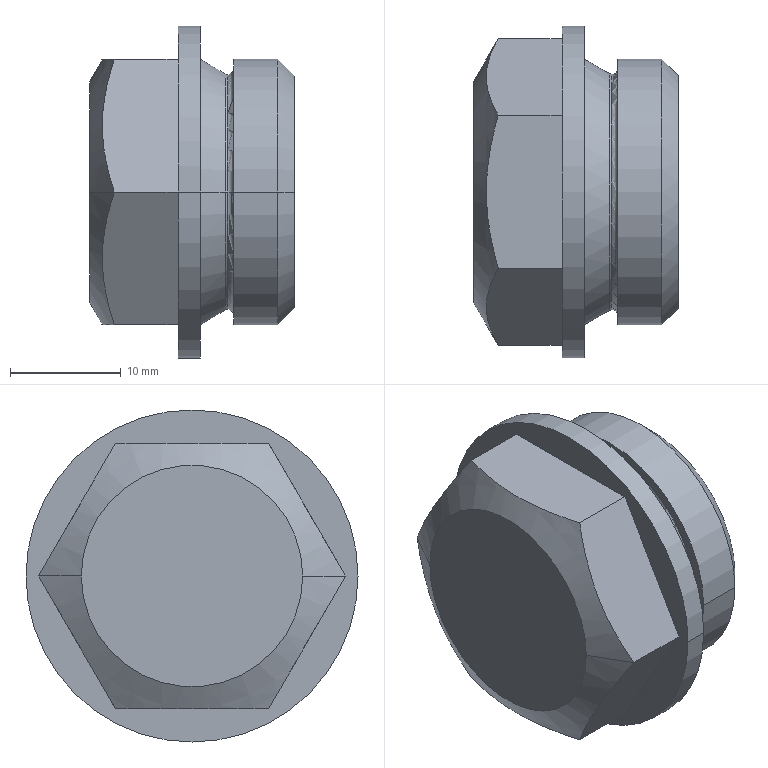Part | SolidWorks | features BaseBody 1 | 1 solid | 28 faces | box 18.5 x 30 x 30 mm | volume 4753 mm3 | plane 12 | cylinder 6 | cone 6 | torus 4 | commonest cylinder face diameters 17.5 x2 24 x2 30 x2
STEP:
#1=CARTESIAN_POINT('',(0.75,87.299,-16.));
#2=VERTEX_POINT('',#1);
#3=CARTESIAN_POINT('',(1.,87.366,-16.));
#4=VERTEX_POINT('',#3);
#5=CARTESIAN_POINT('',(1.,86.866,-16.));
#6=DIRECTION('',(0.,0.,-1.));
#7=DIRECTION('',(0.,1.,0.));
#8=AXIS2_PLACEMENT_3D('',#5,#6,#7);
#9=CIRCLE('',#8,0.5);
#10=EDGE_CURVE('',#2,#4,#9,.T.);
#11=ORIENTED_EDGE('',*,*,#10,.T.);
#12=CARTESIAN_POINT('',(1.,108.634,-16.));
#13=VERTEX_POINT('',#12);
#14=CARTESIAN_POINT('',(1.,98.,-16.));
#15=DIRECTION('',(-1.,0.,0.));
#16=DIRECTION('',(0.,-1.,0.));
#17=AXIS2_PLACEMENT_3D('',#14,#15,#16);
#18=CIRCLE('',#17,10.634);
#19=EDGE_CURVE('',#4,#13,#18,.T.);
#20=ORIENTED_EDGE('',*,*,#19,.T.);
#21=CARTESIAN_POINT('',(0.75,108.701,-16.));
#22=VERTEX_POINT('',#21);
#23=CARTESIAN_POINT('',(1.,109.134,-16.));
#24=DIRECTION('',(0.,0.,1.));
#25=DIRECTION('',(0.,-1.,0.));
#26=AXIS2_PLACEMENT_3D('',#23,#24,#25);
#27=CIRCLE('',#26,0.5);
#28=EDGE_CURVE('',#22,#13,#27,.T.);
#29=ORIENTED_EDGE('',*,*,#28,.F.);
#30=CARTESIAN_POINT('',(0.75,98.,-16.));
#31=DIRECTION('',(-1.,0.,0.));
#32=DIRECTION('',(0.,-1.,0.));
#33=AXIS2_PLACEMENT_3D('',#30,#31,#32);
#34=CIRCLE('',#33,10.701);
#35=EDGE_CURVE('',#2,#22,#34,.T.);
#36=ORIENTED_EDGE('',*,*,#35,.F.);
#37=EDGE_LOOP('',(#11,#20,#29,#36));
#38=FACE_OUTER_BOUND('',#37,.T.);
#39=CARTESIAN_POINT('',(1.,98.,-16.));
#40=DIRECTION('',(-1.,0.,0.));
#41=DIRECTION('',(0.,-1.,0.));
#42=AXIS2_PLACEMENT_3D('',#39,#40,#41);
#43=TOROIDAL_SURFACE('',#42,11.134,0.5);
#44=ADVANCED_FACE('',(#38),#43,.F.);
#45=ORIENTED_EDGE('',*,*,#28,.T.);
#46=CARTESIAN_POINT('',(1.,98.,-16.));
#47=DIRECTION('',(-1.,0.,0.));
#48=DIRECTION('',(0.,-1.,0.));
#49=AXIS2_PLACEMENT_3D('',#46,#47,#48);
#50=CIRCLE('',#49,10.634);
#51=EDGE_CURVE('',#13,#4,#50,.T.);
#52=ORIENTED_EDGE('',*,*,#51,.T.);
#53=ORIENTED_EDGE('',*,*,#10,.F.);
#54=CARTESIAN_POINT('',(0.75,98.,-16.));
#55=DIRECTION('',(-1.,0.,0.));
#56=DIRECTION('',(0.,-1.,0.));
#57=AXIS2_PLACEMENT_3D('',#54,#55,#56);
#58=CIRCLE('',#57,10.701);
#59=EDGE_CURVE('',#22,#2,#58,.T.);
#60=ORIENTED_EDGE('',*,*,#59,.F.);
#61=EDGE_LOOP('',(#45,#52,#53,#60));
#62=FACE_OUTER_BOUND('',#61,.T.);
#63=CARTESIAN_POINT('',(1.,98.,-16.));
#64=DIRECTION('',(-1.,0.,0.));
#65=DIRECTION('',(0.,-1.,0.));
#66=AXIS2_PLACEMENT_3D('',#63,#64,#65);
#67=TOROIDAL_SURFACE('',#66,11.134,0.5);
#68=ADVANCED_FACE('',(#62),#67,.F.);
#69=CARTESIAN_POINT('',(-10.,89.25,-16.));
#70=VERTEX_POINT('',#69);
#71=CARTESIAN_POINT('',(-10.,106.75,-16.));
#72=VERTEX_POINT('',#71);
#73=CARTESIAN_POINT('',(-10.,98.,-16.));
#74=DIRECTION('',(1.,0.,0.));
#75=DIRECTION('',(0.,1.,0.));
#76=AXIS2_PLACEMENT_3D('',#73,#74,#75);
#77=CIRCLE('',#76,8.75);
#78=EDGE_CURVE('',#70,#72,#77,.T.);
#79=ORIENTED_EDGE('',*,*,#78,.F.);
#80=CARTESIAN_POINT('',(7.,89.25,-16.));
#81=VERTEX_POINT('',#80);
#82=CARTESIAN_POINT('',(-10.,89.25,-16.));
#83=DIRECTION('',(1.,0.,0.));
#84=VECTOR('',#83,1000.);
#85=LINE('',#82,#84);
#86=EDGE_CURVE('',#70,#81,#85,.T.);
#87=ORIENTED_EDGE('',*,*,#86,.T.);
#88=CARTESIAN_POINT('',(7.,106.75,-16.));
#89=VERTEX_POINT('',#88);
#90=CARTESIAN_POINT('',(7.,98.,-16.));
#91=DIRECTION('',(1.,0.,0.));
#92=DIRECTION('',(0.,1.,0.));
#93=AXIS2_PLACEMENT_3D('',#90,#91,#92);
#94=CIRCLE('',#93,8.75);
#95=EDGE_CURVE('',#81,#89,#94,.T.);
#96=ORIENTED_EDGE('',*,*,#95,.T.);
#97=CARTESIAN_POINT('',(-10.,106.75,-16.));
#98=DIRECTION('',(1.,0.,0.));
#99=VECTOR('',#98,1000.);
#100=LINE('',#97,#99);
#101=EDGE_CURVE('',#72,#89,#100,.T.);
#102=ORIENTED_EDGE('',*,*,#101,.F.);
#103=EDGE_LOOP('',(#79,#87,#96,#102));
#104=FACE_OUTER_BOUND('',#103,.T.);
#105=CARTESIAN_POINT('',(-10.,98.,-16.));
#106=DIRECTION('',(1.,0.,0.));
#107=DIRECTION('',(0.,1.,0.));
#108=AXIS2_PLACEMENT_3D('',#105,#106,#107);
#109=CYLINDRICAL_SURFACE('',#108,8.75);
#110=ADVANCED_FACE('',(#104),#109,.F.);
#111=CARTESIAN_POINT('',(-11.5,108.,-16.));
#112=VERTEX_POINT('',#111);
#113=CARTESIAN_POINT('',(-11.5,88.,-16.));
#114=VERTEX_POINT('',#113);
#115=CARTESIAN_POINT('',(-11.5,98.,-16.));
#116=DIRECTION('',(-1.,0.,0.));
#117=DIRECTION('',(0.,-1.,0.));
#118=AXIS2_PLACEMENT_3D('',#115,#116,#117);
#119=CIRCLE('',#118,10.);
#120=EDGE_CURVE('',#112,#114,#119,.T.);
#121=ORIENTED_EDGE('',*,*,#120,.F.);
#122=CARTESIAN_POINT('',(-9.274,111.856,-16.));
#123=VERTEX_POINT('',#122);
#124=CARTESIAN_POINT('',(-11.5,108.,-16.));
#125=DIRECTION('',(0.5,0.866,0.));
#126=VECTOR('',#125,1000.);
#127=LINE('',#124,#126);
#128=EDGE_CURVE('',#112,#123,#127,.T.);
#129=ORIENTED_EDGE('',*,*,#128,.T.);
#130=CARTESIAN_POINT('',(-9.274,104.928,-28.));
#131=VERTEX_POINT('',#130);
#132=CARTESIAN_POINT('',(-9.274,111.856,-16.));
#133=CARTESIAN_POINT('',(-9.6,111.291,-16.98));
#134=CARTESIAN_POINT('',(-9.869,110.721,-17.967));
#135=CARTESIAN_POINT('',(-10.242,109.57,-19.961));
#136=CARTESIAN_POINT('',(-10.345,108.988,-20.968));
#137=CARTESIAN_POINT('',(-10.346,108.104,-22.499));
#138=CARTESIAN_POINT('',(-10.321,107.809,-23.011));
#139=CARTESIAN_POINT('',(-10.223,107.223,-24.025));
#140=CARTESIAN_POINT('',(-10.15,106.933,-24.528));
#141=CARTESIAN_POINT('',(-9.87,106.066,-26.03));
#142=CARTESIAN_POINT('',(-9.6,105.495,-27.019));
#143=CARTESIAN_POINT('',(-9.274,104.928,-28.));
#144=B_SPLINE_CURVE_WITH_KNOTS('',3,(#132,#133,#134,#135,#136,#137,#138,#139,#140,#141,#142,#143),.UNSPECIFIED.,.F.,.F.,(4,2,2,2,2,4),(0.000000238,0.003499,0.006997,0.008747,0.0105,0.01399),.UNSPECIFIED.);
#145=EDGE_CURVE('',#123,#131,#144,.T.);
#146=ORIENTED_EDGE('',*,*,#145,.T.);
#147=CARTESIAN_POINT('',(-9.274,91.072,-28.));
#148=VERTEX_POINT('',#147);
#149=CARTESIAN_POINT('',(-9.274,104.928,-28.));
#150=CARTESIAN_POINT('',(-9.597,103.808,-28.));
#151=CARTESIAN_POINT('',(-9.866,102.674,-28.));
#152=CARTESIAN_POINT('',(-10.148,100.939,-28.));
#153=CARTESIAN_POINT('',(-10.221,100.355,-28.));
#154=CARTESIAN_POINT('',(-10.32,99.176,-28.));
#155=CARTESIAN_POINT('',(-10.345,98.588,-28.));
#156=CARTESIAN_POINT('',(-10.345,96.831,-28.));
#157=CARTESIAN_POINT('',(-10.245,95.667,-28.));
#158=CARTESIAN_POINT('',(-9.872,93.354,-28.));
#159=CARTESIAN_POINT('',(-9.599,92.199,-28.));
#160=CARTESIAN_POINT('',(-9.274,91.072,-28.));
#161=B_SPLINE_CURVE_WITH_KNOTS('',3,(#149,#150,#151,#152,#153,#154,#155,#156,#157,#158,#159,#160),.UNSPECIFIED.,.F.,.F.,(4,2,2,2,2,4),(0.004977,0.008474,0.01022,0.01197,0.01547,0.01896),.UNSPECIFIED.);
#162=EDGE_CURVE('',#131,#148,#161,.T.);
#163=ORIENTED_EDGE('',*,*,#162,.T.);
#164=CARTESIAN_POINT('',(-9.274,84.144,-16.));
#165=VERTEX_POINT('',#164);
#166=CARTESIAN_POINT('',(-9.274,91.072,-28.));
#167=CARTESIAN_POINT('',(-9.6,90.506,-27.02));
#168=CARTESIAN_POINT('',(-9.869,89.936,-26.033));
#169=CARTESIAN_POINT('',(-10.242,88.785,-24.039));
#170=CARTESIAN_POINT('',(-10.345,88.203,-23.032));
#171=CARTESIAN_POINT('',(-10.346,87.32,-21.501));
#172=CARTESIAN_POINT('',(-10.321,87.024,-20.989));
#173=CARTESIAN_POINT('',(-10.223,86.439,-19.975));
#174=CARTESIAN_POINT('',(-10.15,86.148,-19.472));
#175=CARTESIAN_POINT('',(-9.87,85.281,-17.97));
#176=CARTESIAN_POINT('',(-9.6,84.71,-16.981));
#177=CARTESIAN_POINT('',(-9.274,84.144,-16.));
#178=B_SPLINE_CURVE_WITH_KNOTS('',3,(#166,#167,#168,#169,#170,#171,#172,#173,#174,#175,#176,#177),.UNSPECIFIED.,.F.,.F.,(4,2,2,2,2,4),(0.000000238,0.003499,0.006997,0.008747,0.0105,0.01399),.UNSPECIFIED.);
#179=EDGE_CURVE('',#148,#165,#178,.T.);
#180=ORIENTED_EDGE('',*,*,#179,.T.);
#181=CARTESIAN_POINT('',(-11.5,88.,-16.));
#182=DIRECTION('',(0.5,-0.866,0.));
#183=VECTOR('',#182,1000.);
#184=LINE('',#181,#183);
#185=EDGE_CURVE('',#114,#165,#184,.T.);
#186=ORIENTED_EDGE('',*,*,#185,.F.);
#187=EDGE_LOOP('',(#121,#129,#146,#163,#180,#186));
#188=FACE_OUTER_BOUND('',#187,.T.);
#189=CARTESIAN_POINT('',(-11.5,98.,-16.));
#190=DIRECTION('',(1.,0.,0.));
#191=DIRECTION('',(0.,-1.,0.));
#192=AXIS2_PLACEMENT_3D('',#189,#190,#191);
#193=CONICAL_SURFACE('',#192,10.,1.047);
#194=ADVANCED_FACE('',(#188),#193,.T.);
#195=ORIENTED_EDGE('',*,*,#51,.F.);
#196=CARTESIAN_POINT('',(1.5,109.134,-16.));
#197=VERTEX_POINT('',#196);
#198=CARTESIAN_POINT('',(1.,109.134,-16.));
#199=DIRECTION('',(0.,0.,1.));
#200=DIRECTION('',(0.,-1.,0.));
#201=AXIS2_PLACEMENT_3D('',#198,#199,#200);
#202=CIRCLE('',#201,0.5);
#203=EDGE_CURVE('',#13,#197,#202,.T.);
#204=ORIENTED_EDGE('',*,*,#203,.T.);
#205=CARTESIAN_POINT('',(1.5,86.866,-16.));
#206=VERTEX_POINT('',#205);
#207=CARTESIAN_POINT('',(1.5,98.,-16.));
#208=DIRECTION('',(-1.,0.,0.));
#209=DIRECTION('',(0.,-1.,0.));
#210=AXIS2_PLACEMENT_3D('',#207,#208,#209);
#211=CIRCLE('',#210,11.134);
#212=EDGE_CURVE('',#197,#206,#211,.T.);
#213=ORIENTED_EDGE('',*,*,#212,.T.);
#214=CARTESIAN_POINT('',(1.,86.866,-16.));
#215=DIRECTION('',(0.,0.,-1.));
#216=DIRECTION('',(0.,1.,0.));
#217=AXIS2_PLACEMENT_3D('',#214,#215,#216);
#218=CIRCLE('',#217,0.5);
#219=EDGE_CURVE('',#4,#206,#218,.T.);
#220=ORIENTED_EDGE('',*,*,#219,.F.);
#221=EDGE_LOOP('',(#195,#204,#213,#220));
#222=FACE_OUTER_BOUND('',#221,.T.);
#223=CARTESIAN_POINT('',(1.,98.,-16.));
#224=DIRECTION('',(-1.,0.,0.));
#225=DIRECTION('',(0.,-1.,0.));
#226=AXIS2_PLACEMENT_3D('',#223,#224,#225);
#227=TOROIDAL_SURFACE('',#226,11.134,0.5);
#228=ADVANCED_FACE('',(#222),#227,.F.);
#229=ORIENTED_EDGE('',*,*,#35,.T.);
#230=CARTESIAN_POINT('',(-1.5,110.,-16.));
#231=VERTEX_POINT('',#230);
#232=CARTESIAN_POINT('',(-1.5,110.,-16.));
#233=DIRECTION('',(-0.866,0.5,0.));
#234=VECTOR('',#233,1000.);
#235=LINE('',#232,#234);
#236=EDGE_CURVE('',#22,#231,#235,.T.);
#237=ORIENTED_EDGE('',*,*,#236,.T.);
#238=CARTESIAN_POINT('',(-1.5,86.,-16.));
#239=VERTEX_POINT('',#238);
#240=CARTESIAN_POINT('',(-1.5,98.,-16.));
#241=DIRECTION('',(-1.,0.,0.));
#242=DIRECTION('',(0.,-1.,0.));
#243=AXIS2_PLACEMENT_3D('',#240,#241,#242);
#244=CIRCLE('',#243,12.);
#245=EDGE_CURVE('',#239,#231,#244,.T.);
#246=ORIENTED_EDGE('',*,*,#245,.F.);
#247=CARTESIAN_POINT('',(-1.5,86.,-16.));
#248=DIRECTION('',(-0.866,-0.5,0.));
#249=VECTOR('',#248,1000.);
#250=LINE('',#247,#249);
#251=EDGE_CURVE('',#2,#239,#250,.T.);
#252=ORIENTED_EDGE('',*,*,#251,.F.);
#253=EDGE_LOOP('',(#229,#237,#246,#252));
#254=FACE_OUTER_BOUND('',#253,.T.);
#255=CARTESIAN_POINT('',(-1.5,98.,-16.));
#256=DIRECTION('',(-1.,0.,0.));
#257=DIRECTION('',(0.,-1.,0.));
#258=AXIS2_PLACEMENT_3D('',#255,#256,#257);
#259=CONICAL_SURFACE('',#258,12.,0.5236);
#260=ADVANCED_FACE('',(#254),#259,.T.);
#261=CARTESIAN_POINT('',(7.,87.5,-16.));
#262=VERTEX_POINT('',#261);
#263=CARTESIAN_POINT('',(7.,108.5,-16.));
#264=VERTEX_POINT('',#263);
#265=CARTESIAN_POINT('',(7.,98.,-16.));
#266=DIRECTION('',(-1.,0.,0.));
#267=DIRECTION('',(0.,-1.,0.));
#268=AXIS2_PLACEMENT_3D('',#265,#266,#267);
#269=CIRCLE('',#268,10.5);
#270=EDGE_CURVE('',#262,#264,#269,.T.);
#271=ORIENTED_EDGE('',*,*,#270,.T.);
#272=CARTESIAN_POINT('',(5.5,110.,-16.));
#273=VERTEX_POINT('',#272);
#274=CARTESIAN_POINT('',(5.5,110.,-16.));
#275=DIRECTION('',(-0.7071,0.7071,0.));
#276=VECTOR('',#275,1000.);
#277=LINE('',#274,#276);
#278=EDGE_CURVE('',#264,#273,#277,.T.);
#279=ORIENTED_EDGE('',*,*,#278,.T.);
#280=CARTESIAN_POINT('',(5.5,86.,-16.));
#281=VERTEX_POINT('',#280);
#282=CARTESIAN_POINT('',(5.5,98.,-16.));
#283=DIRECTION('',(-1.,0.,0.));
#284=DIRECTION('',(0.,-1.,0.));
#285=AXIS2_PLACEMENT_3D('',#282,#283,#284);
#286=CIRCLE('',#285,12.);
#287=EDGE_CURVE('',#281,#273,#286,.T.);
#288=ORIENTED_EDGE('',*,*,#287,.F.);
#289=CARTESIAN_POINT('',(5.5,86.,-16.));
#290=DIRECTION('',(-0.7071,-0.7071,0.));
#291=VECTOR('',#290,1000.);
#292=LINE('',#289,#291);
#293=EDGE_CURVE('',#262,#281,#292,.T.);
#294=ORIENTED_EDGE('',*,*,#293,.F.);
#295=EDGE_LOOP('',(#271,#279,#288,#294));
#296=FACE_OUTER_BOUND('',#295,.T.);
#297=CARTESIAN_POINT('',(5.5,98.,-16.));
#298=DIRECTION('',(-1.,0.,0.));
#299=DIRECTION('',(0.,-1.,0.));
#300=AXIS2_PLACEMENT_3D('',#297,#298,#299);
#301=CONICAL_SURFACE('',#300,12.,0.7854);
#302=ADVANCED_FACE('',(#296),#301,.T.);
#303=ORIENTED_EDGE('',*,*,#287,.T.);
#304=CARTESIAN_POINT('',(1.5,110.,-16.));
#305=VERTEX_POINT('',#304);
#306=CARTESIAN_POINT('',(-11.5,110.,-16.));
#307=DIRECTION('',(-1.,0.,0.));
#308=VECTOR('',#307,1000.);
#309=LINE('',#306,#308);
#310=EDGE_CURVE('',#273,#305,#309,.T.);
#311=ORIENTED_EDGE('',*,*,#310,.T.);
#312=CARTESIAN_POINT('',(1.5,86.,-16.));
#313=VERTEX_POINT('',#312);
#314=CARTESIAN_POINT('',(1.5,98.,-16.));
#315=DIRECTION('',(-1.,0.,0.));
#316=DIRECTION('',(0.,-1.,0.));
#317=AXIS2_PLACEMENT_3D('',#314,#315,#316);
#318=CIRCLE('',#317,12.);
#319=EDGE_CURVE('',#313,#305,#318,.T.);
#320=ORIENTED_EDGE('',*,*,#319,.F.);
#321=CARTESIAN_POINT('',(-11.5,86.,-16.));
#322=DIRECTION('',(-1.,0.,0.));
#323=VECTOR('',#322,1000.);
#324=LINE('',#321,#323);
#325=EDGE_CURVE('',#281,#313,#324,.T.);
#326=ORIENTED_EDGE('',*,*,#325,.F.);
#327=EDGE_LOOP('',(#303,#311,#320,#326));
#328=FACE_OUTER_BOUND('',#327,.T.);
#329=CARTESIAN_POINT('',(-11.5,98.,-16.));
#330=DIRECTION('',(-1.,0.,0.));
#331=DIRECTION('',(0.,-1.,0.));
#332=AXIS2_PLACEMENT_3D('',#329,#330,#331);
#333=CYLINDRICAL_SURFACE('',#332,12.);
#334=ADVANCED_FACE('',(#328),#333,.T.);
#335=CARTESIAN_POINT('',(-3.5,113.,-16.));
#336=VERTEX_POINT('',#335);
#337=CARTESIAN_POINT('',(-3.5,83.,-16.));
#338=VERTEX_POINT('',#337);
#339=CARTESIAN_POINT('',(-3.5,98.,-16.));
#340=DIRECTION('',(1.,0.,0.));
#341=DIRECTION('',(0.,1.,0.));
#342=AXIS2_PLACEMENT_3D('',#339,#340,#341);
#343=CIRCLE('',#342,15.);
#344=EDGE_CURVE('',#336,#338,#343,.T.);
#345=ORIENTED_EDGE('',*,*,#344,.T.);
#346=CARTESIAN_POINT('',(-1.5,83.,-16.));
#347=VERTEX_POINT('',#346);
#348=CARTESIAN_POINT('',(-3.5,83.,-16.));
#349=DIRECTION('',(1.,0.,0.));
#350=VECTOR('',#349,1000.);
#351=LINE('',#348,#350);
#352=EDGE_CURVE('',#338,#347,#351,.T.);
#353=ORIENTED_EDGE('',*,*,#352,.T.);
#354=CARTESIAN_POINT('',(-1.5,113.,-16.));
#355=VERTEX_POINT('',#354);
#356=CARTESIAN_POINT('',(-1.5,98.,-16.));
#357=DIRECTION('',(1.,0.,0.));
#358=DIRECTION('',(0.,1.,0.));
#359=AXIS2_PLACEMENT_3D('',#356,#357,#358);
#360=CIRCLE('',#359,15.);
#361=EDGE_CURVE('',#355,#347,#360,.T.);
#362=ORIENTED_EDGE('',*,*,#361,.F.);
#363=CARTESIAN_POINT('',(-3.5,113.,-16.));
#364=DIRECTION('',(1.,0.,0.));
#365=VECTOR('',#364,1000.);
#366=LINE('',#363,#365);
#367=EDGE_CURVE('',#336,#355,#366,.T.);
#368=ORIENTED_EDGE('',*,*,#367,.F.);
#369=EDGE_LOOP('',(#345,#353,#362,#368));
#370=FACE_OUTER_BOUND('',#369,.T.);
#371=CARTESIAN_POINT('',(-3.5,98.,-16.));
#372=DIRECTION('',(1.,0.,0.));
#373=DIRECTION('',(0.,1.,0.));
#374=AXIS2_PLACEMENT_3D('',#371,#372,#373);
#375=CYLINDRICAL_SURFACE('',#374,15.);
#376=ADVANCED_FACE('',(#370),#375,.T.);
#377=ORIENTED_EDGE('',*,*,#145,.F.);
#378=CARTESIAN_POINT('',(-3.5,111.856,-16.));
#379=VERTEX_POINT('',#378);
#380=CARTESIAN_POINT('',(-1.5,111.856,-16.));
#381=DIRECTION('',(-1.,0.,0.));
#382=VECTOR('',#381,1000.);
#383=LINE('',#380,#382);
#384=EDGE_CURVE('',#379,#123,#383,.T.);
#385=ORIENTED_EDGE('',*,*,#384,.F.);
#386=CARTESIAN_POINT('',(-3.5,104.928,-28.));
#387=VERTEX_POINT('',#386);
#388=CARTESIAN_POINT('',(-3.5,104.928,-28.));
#389=DIRECTION('',(0.,0.5,0.866));
#390=VECTOR('',#389,1000.);
#391=LINE('',#388,#390);
#392=EDGE_CURVE('',#387,#379,#391,.T.);
#393=ORIENTED_EDGE('',*,*,#392,.F.);
#394=CARTESIAN_POINT('',(-1.5,104.928,-28.));
#395=DIRECTION('',(-1.,0.,0.));
#396=VECTOR('',#395,1000.);
#397=LINE('',#394,#396);
#398=EDGE_CURVE('',#387,#131,#397,.T.);
#399=ORIENTED_EDGE('',*,*,#398,.T.);
#400=EDGE_LOOP('',(#377,#385,#393,#399));
#401=FACE_OUTER_BOUND('',#400,.T.);
#402=CARTESIAN_POINT('',(-1.5,104.928,-28.));
#403=DIRECTION('',(0.,-0.866,0.5));
#404=DIRECTION('',(0.,-0.5,-0.866));
#405=AXIS2_PLACEMENT_3D('',#402,#403,#404);
#406=PLANE('',#405);
#407=ADVANCED_FACE('',(#401),#406,.F.);
#408=CARTESIAN_POINT('',(-9.274,104.928,-4.));
#409=VERTEX_POINT('',#408);
#410=CARTESIAN_POINT('',(-9.274,104.928,-4.));
#411=CARTESIAN_POINT('',(-9.6,105.494,-4.98));
#412=CARTESIAN_POINT('',(-9.869,106.064,-5.967));
#413=CARTESIAN_POINT('',(-10.242,107.215,-7.961));
#414=CARTESIAN_POINT('',(-10.345,107.797,-8.968));
#415=CARTESIAN_POINT('',(-10.346,108.68,-10.499));
#416=CARTESIAN_POINT('',(-10.321,108.976,-11.011));
#417=CARTESIAN_POINT('',(-10.223,109.561,-12.025));
#418=CARTESIAN_POINT('',(-10.15,109.852,-12.528));
#419=CARTESIAN_POINT('',(-9.87,110.719,-14.03));
#420=CARTESIAN_POINT('',(-9.6,111.29,-15.019));
#421=CARTESIAN_POINT('',(-9.274,111.856,-16.));
#422=B_SPLINE_CURVE_WITH_KNOTS('',3,(#410,#411,#412,#413,#414,#415,#416,#417,#418,#419,#420,#421),.UNSPECIFIED.,.F.,.F.,(4,2,2,2,2,4),(0.000000238,0.003499,0.006997,0.008747,0.0105,0.01399),.UNSPECIFIED.);
#423=EDGE_CURVE('',#409,#123,#422,.T.);
#424=ORIENTED_EDGE('',*,*,#423,.F.);
#425=CARTESIAN_POINT('',(-3.5,104.928,-4.));
#426=VERTEX_POINT('',#425);
#427=CARTESIAN_POINT('',(-1.5,104.928,-4.));
#428=DIRECTION('',(-1.,0.,0.));
#429=VECTOR('',#428,1000.);
#430=LINE('',#427,#429);
#431=EDGE_CURVE('',#426,#409,#430,.T.);
#432=ORIENTED_EDGE('',*,*,#431,.F.);
#433=CARTESIAN_POINT('',(-3.5,104.928,-4.));
#434=DIRECTION('',(0.,-0.5,0.866));
#435=VECTOR('',#434,1000.);
#436=LINE('',#433,#435);
#437=EDGE_CURVE('',#379,#426,#436,.T.);
#438=ORIENTED_EDGE('',*,*,#437,.F.);
#439=ORIENTED_EDGE('',*,*,#384,.T.);
#440=EDGE_LOOP('',(#424,#432,#438,#439));
#441=FACE_OUTER_BOUND('',#440,.T.);
#442=CARTESIAN_POINT('',(-1.5,104.928,-4.));
#443=DIRECTION('',(0.,-0.866,-0.5));
#444=DIRECTION('',(0.,0.5,-0.866));
#445=AXIS2_PLACEMENT_3D('',#442,#443,#444);
#446=PLANE('',#445);
#447=ADVANCED_FACE('',(#441),#446,.F.);
#448=CARTESIAN_POINT('',(-9.274,91.072,-4.));
#449=VERTEX_POINT('',#448);
#450=CARTESIAN_POINT('',(-9.274,91.072,-4.));
#451=CARTESIAN_POINT('',(-9.599,92.199,-4.));
#452=CARTESIAN_POINT('',(-9.872,93.354,-4.));
#453=CARTESIAN_POINT('',(-10.245,95.667,-4.));
#454=CARTESIAN_POINT('',(-10.345,96.831,-4.));
#455=CARTESIAN_POINT('',(-10.345,98.588,-4.));
#456=CARTESIAN_POINT('',(-10.32,99.176,-4.));
#457=CARTESIAN_POINT('',(-10.221,100.355,-4.));
#458=CARTESIAN_POINT('',(-10.148,100.939,-4.));
#459=CARTESIAN_POINT('',(-9.866,102.674,-4.));
#460=CARTESIAN_POINT('',(-9.597,103.808,-4.));
#461=CARTESIAN_POINT('',(-9.274,104.928,-4.));
#462=B_SPLINE_CURVE_WITH_KNOTS('',3,(#450,#451,#452,#453,#454,#455,#456,#457,#458,#459,#460,#461),.UNSPECIFIED.,.F.,.F.,(4,2,2,2,2,4),(0.01246,0.01596,0.01947,0.02122,0.02297,0.02648),.UNSPECIFIED.);
#463=EDGE_CURVE('',#449,#409,#462,.T.);
#464=ORIENTED_EDGE('',*,*,#463,.F.);
#465=CARTESIAN_POINT('',(-3.5,91.072,-4.));
#466=VERTEX_POINT('',#465);
#467=CARTESIAN_POINT('',(-1.5,91.072,-4.));
#468=DIRECTION('',(-1.,0.,0.));
#469=VECTOR('',#468,1000.);
#470=LINE('',#467,#469);
#471=EDGE_CURVE('',#466,#449,#470,.T.);
#472=ORIENTED_EDGE('',*,*,#471,.F.);
#473=CARTESIAN_POINT('',(-3.5,91.072,-4.));
#474=DIRECTION('',(0.,-1.,0.));
#475=VECTOR('',#474,1000.);
#476=LINE('',#473,#475);
#477=EDGE_CURVE('',#426,#466,#476,.T.);
#478=ORIENTED_EDGE('',*,*,#477,.F.);
#479=ORIENTED_EDGE('',*,*,#431,.T.);
#480=EDGE_LOOP('',(#464,#472,#478,#479));
#481=FACE_OUTER_BOUND('',#480,.T.);
#482=CARTESIAN_POINT('',(-1.5,91.072,-4.));
#483=DIRECTION('',(0.,0.,-1.));
#484=DIRECTION('',(-1.,0.,0.));
#485=AXIS2_PLACEMENT_3D('',#482,#483,#484);
#486=PLANE('',#485);
#487=ADVANCED_FACE('',(#481),#486,.F.);
#488=CARTESIAN_POINT('',(-9.274,84.144,-16.));
#489=CARTESIAN_POINT('',(-9.6,84.709,-15.02));
#490=CARTESIAN_POINT('',(-9.869,85.279,-14.033));
#491=CARTESIAN_POINT('',(-10.242,86.43,-12.039));
#492=CARTESIAN_POINT('',(-10.345,87.012,-11.032));
#493=CARTESIAN_POINT('',(-10.346,87.896,-9.501));
#494=CARTESIAN_POINT('',(-10.321,88.191,-8.989));
#495=CARTESIAN_POINT('',(-10.223,88.777,-7.975));
#496=CARTESIAN_POINT('',(-10.15,89.067,-7.472));
#497=CARTESIAN_POINT('',(-9.87,89.934,-5.97));
#498=CARTESIAN_POINT('',(-9.6,90.505,-4.981));
#499=CARTESIAN_POINT('',(-9.274,91.072,-4.));
#500=B_SPLINE_CURVE_WITH_KNOTS('',3,(#488,#489,#490,#491,#492,#493,#494,#495,#496,#497,#498,#499),.UNSPECIFIED.,.F.,.F.,(4,2,2,2,2,4),(0.000000238,0.003499,0.006997,0.008747,0.0105,0.01399),.UNSPECIFIED.);
#501=EDGE_CURVE('',#165,#449,#500,.T.);
#502=ORIENTED_EDGE('',*,*,#501,.F.);
#503=CARTESIAN_POINT('',(-3.5,84.144,-16.));
#504=VERTEX_POINT('',#503);
#505=CARTESIAN_POINT('',(-1.5,84.144,-16.));
#506=DIRECTION('',(-1.,0.,0.));
#507=VECTOR('',#506,1000.);
#508=LINE('',#505,#507);
#509=EDGE_CURVE('',#504,#165,#508,.T.);
#510=ORIENTED_EDGE('',*,*,#509,.F.);
#511=CARTESIAN_POINT('',(-3.5,91.072,-4.));
#512=DIRECTION('',(0.,-0.5,-0.866));
#513=VECTOR('',#512,1000.);
#514=LINE('',#511,#513);
#515=EDGE_CURVE('',#466,#504,#514,.T.);
#516=ORIENTED_EDGE('',*,*,#515,.F.);
#517=ORIENTED_EDGE('',*,*,#471,.T.);
#518=EDGE_LOOP('',(#502,#510,#516,#517));
#519=FACE_OUTER_BOUND('',#518,.T.);
#520=CARTESIAN_POINT('',(-1.5,91.072,-4.));
#521=DIRECTION('',(0.,0.866,-0.5));
#522=DIRECTION('',(0.,0.5,0.866));
#523=AXIS2_PLACEMENT_3D('',#520,#521,#522);
#524=PLANE('',#523);
#525=ADVANCED_FACE('',(#519),#524,.F.);
#526=ORIENTED_EDGE('',*,*,#179,.F.);
#527=CARTESIAN_POINT('',(-3.5,91.072,-28.));
#528=VERTEX_POINT('',#527);
#529=CARTESIAN_POINT('',(-1.5,91.072,-28.));
#530=DIRECTION('',(-1.,0.,0.));
#531=VECTOR('',#530,1000.);
#532=LINE('',#529,#531);
#533=EDGE_CURVE('',#528,#148,#532,.T.);
#534=ORIENTED_EDGE('',*,*,#533,.F.);
#535=CARTESIAN_POINT('',(-3.5,91.072,-28.));
#536=DIRECTION('',(0.,0.5,-0.866));
#537=VECTOR('',#536,1000.);
#538=LINE('',#535,#537);
#539=EDGE_CURVE('',#504,#528,#538,.T.);
#540=ORIENTED_EDGE('',*,*,#539,.F.);
#541=ORIENTED_EDGE('',*,*,#509,.T.);
#542=EDGE_LOOP('',(#526,#534,#540,#541));
#543=FACE_OUTER_BOUND('',#542,.T.);
#544=CARTESIAN_POINT('',(-1.5,91.072,-28.));
#545=DIRECTION('',(0.,0.866,0.5));
#546=DIRECTION('',(0.,-0.5,0.866));
#547=AXIS2_PLACEMENT_3D('',#544,#545,#546);
#548=PLANE('',#547);
#549=ADVANCED_FACE('',(#543),#548,.F.);
#550=ORIENTED_EDGE('',*,*,#162,.F.);
#551=ORIENTED_EDGE('',*,*,#398,.F.);
#552=CARTESIAN_POINT('',(-3.5,91.072,-28.));
#553=DIRECTION('',(0.,1.,0.));
#554=VECTOR('',#553,1000.);
#555=LINE('',#552,#554);
#556=EDGE_CURVE('',#528,#387,#555,.T.);
#557=ORIENTED_EDGE('',*,*,#556,.F.);
#558=ORIENTED_EDGE('',*,*,#533,.T.);
#559=EDGE_LOOP('',(#550,#551,#557,#558));
#560=FACE_OUTER_BOUND('',#559,.T.);
#561=CARTESIAN_POINT('',(-1.5,91.072,-28.));
#562=DIRECTION('',(0.,0.,1.));
#563=DIRECTION('',(1.,0.,0.));
#564=AXIS2_PLACEMENT_3D('',#561,#562,#563);
#565=PLANE('',#564);
#566=ADVANCED_FACE('',(#560),#565,.F.);
#567=ORIENTED_EDGE('',*,*,#344,.F.);
#568=CARTESIAN_POINT('',(-3.5,98.,-16.));
#569=DIRECTION('',(1.,0.,0.));
#570=DIRECTION('',(0.,1.,0.));
#571=AXIS2_PLACEMENT_3D('',#568,#569,#570);
#572=CIRCLE('',#571,15.);
#573=EDGE_CURVE('',#338,#336,#572,.T.);
#574=ORIENTED_EDGE('',*,*,#573,.F.);
#575=EDGE_LOOP('',(#567,#574));
#576=FACE_OUTER_BOUND('',#575,.T.);
#577=ORIENTED_EDGE('',*,*,#556,.T.);
#578=ORIENTED_EDGE('',*,*,#392,.T.);
#579=ORIENTED_EDGE('',*,*,#437,.T.);
#580=ORIENTED_EDGE('',*,*,#477,.T.);
#581=ORIENTED_EDGE('',*,*,#515,.T.);
#582=ORIENTED_EDGE('',*,*,#539,.T.);
#583=EDGE_LOOP('',(#577,#578,#579,#580,#581,#582));
#584=FACE_BOUND('',#583,.T.);
#585=CARTESIAN_POINT('',(-3.5,98.,-16.));
#586=DIRECTION('',(1.,0.,0.));
#587=DIRECTION('',(0.,1.,0.));
#588=AXIS2_PLACEMENT_3D('',#585,#586,#587);
#589=PLANE('',#588);
#590=ADVANCED_FACE('',(#576,#584),#589,.F.);
#591=ORIENTED_EDGE('',*,*,#352,.F.);
#592=ORIENTED_EDGE('',*,*,#573,.T.);
#593=ORIENTED_EDGE('',*,*,#367,.T.);
#594=CARTESIAN_POINT('',(-1.5,98.,-16.));
#595=DIRECTION('',(1.,0.,0.));
#596=DIRECTION('',(0.,1.,0.));
#597=AXIS2_PLACEMENT_3D('',#594,#595,#596);
#598=CIRCLE('',#597,15.);
#599=EDGE_CURVE('',#347,#355,#598,.T.);
#600=ORIENTED_EDGE('',*,*,#599,.F.);
#601=EDGE_LOOP('',(#591,#592,#593,#600));
#602=FACE_OUTER_BOUND('',#601,.T.);
#603=CARTESIAN_POINT('',(-3.5,98.,-16.));
#604=DIRECTION('',(1.,0.,0.));
#605=DIRECTION('',(0.,1.,0.));
#606=AXIS2_PLACEMENT_3D('',#603,#604,#605);
#607=CYLINDRICAL_SURFACE('',#606,15.);
#608=ADVANCED_FACE('',(#602),#607,.T.);
#609=ORIENTED_EDGE('',*,*,#245,.T.);
#610=CARTESIAN_POINT('',(-1.5,98.,-16.));
#611=DIRECTION('',(-1.,0.,0.));
#612=DIRECTION('',(0.,-1.,0.));
#613=AXIS2_PLACEMENT_3D('',#610,#611,#612);
#614=CIRCLE('',#613,12.);
#615=EDGE_CURVE('',#231,#239,#614,.T.);
#616=ORIENTED_EDGE('',*,*,#615,.T.);
#617=EDGE_LOOP('',(#609,#616));
#618=FACE_BOUND('',#617,.T.);
#619=ORIENTED_EDGE('',*,*,#361,.T.);
#620=ORIENTED_EDGE('',*,*,#599,.T.);
#621=EDGE_LOOP('',(#619,#620));
#622=FACE_OUTER_BOUND('',#621,.T.);
#623=CARTESIAN_POINT('',(-1.5,111.856,-16.));
#624=DIRECTION('',(-1.,0.,0.));
#625=DIRECTION('',(0.,-1.,0.));
#626=AXIS2_PLACEMENT_3D('',#623,#624,#625);
#627=PLANE('',#626);
#628=ADVANCED_FACE('',(#618,#622),#627,.F.);
#629=ORIENTED_EDGE('',*,*,#319,.T.);
#630=CARTESIAN_POINT('',(1.5,98.,-16.));
#631=DIRECTION('',(-1.,0.,0.));
#632=DIRECTION('',(0.,-1.,0.));
#633=AXIS2_PLACEMENT_3D('',#630,#631,#632);
#634=CIRCLE('',#633,12.);
#635=EDGE_CURVE('',#305,#313,#634,.T.);
#636=ORIENTED_EDGE('',*,*,#635,.T.);
#637=EDGE_LOOP('',(#629,#636));
#638=FACE_OUTER_BOUND('',#637,.T.);
#639=CARTESIAN_POINT('',(1.5,98.,-16.));
#640=DIRECTION('',(-1.,0.,0.));
#641=DIRECTION('',(0.,-1.,0.));
#642=AXIS2_PLACEMENT_3D('',#639,#640,#641);
#643=CIRCLE('',#642,11.134);
#644=EDGE_CURVE('',#206,#197,#643,.T.);
#645=ORIENTED_EDGE('',*,*,#644,.F.);
#646=ORIENTED_EDGE('',*,*,#212,.F.);
#647=EDGE_LOOP('',(#645,#646));
#648=FACE_BOUND('',#647,.T.);
#649=CARTESIAN_POINT('',(1.5,86.,-16.));
#650=DIRECTION('',(-1.,0.,0.));
#651=DIRECTION('',(0.,-1.,0.));
#652=AXIS2_PLACEMENT_3D('',#649,#650,#651);
#653=PLANE('',#652);
#654=ADVANCED_FACE('',(#638,#648),#653,.T.);
#655=ORIENTED_EDGE('',*,*,#310,.F.);
#656=CARTESIAN_POINT('',(5.5,98.,-16.));
#657=DIRECTION('',(-1.,0.,0.));
#658=DIRECTION('',(0.,-1.,0.));
#659=AXIS2_PLACEMENT_3D('',#656,#657,#658);
#660=CIRCLE('',#659,12.);
#661=EDGE_CURVE('',#273,#281,#660,.T.);
#662=ORIENTED_EDGE('',*,*,#661,.T.);
#663=ORIENTED_EDGE('',*,*,#325,.T.);
#664=ORIENTED_EDGE('',*,*,#635,.F.);
#665=EDGE_LOOP('',(#655,#662,#663,#664));
#666=FACE_OUTER_BOUND('',#665,.T.);
#667=CARTESIAN_POINT('',(-11.5,98.,-16.));
#668=DIRECTION('',(-1.,0.,0.));
#669=DIRECTION('',(0.,-1.,0.));
#670=AXIS2_PLACEMENT_3D('',#667,#668,#669);
#671=CYLINDRICAL_SURFACE('',#670,12.);
#672=ADVANCED_FACE('',(#666),#671,.T.);
#673=ORIENTED_EDGE('',*,*,#278,.F.);
#674=CARTESIAN_POINT('',(7.,98.,-16.));
#675=DIRECTION('',(-1.,0.,0.));
#676=DIRECTION('',(0.,-1.,0.));
#677=AXIS2_PLACEMENT_3D('',#674,#675,#676);
#678=CIRCLE('',#677,10.5);
#679=EDGE_CURVE('',#264,#262,#678,.T.);
#680=ORIENTED_EDGE('',*,*,#679,.T.);
#681=ORIENTED_EDGE('',*,*,#293,.T.);
#682=ORIENTED_EDGE('',*,*,#661,.F.);
#683=EDGE_LOOP('',(#673,#680,#681,#682));
#684=FACE_OUTER_BOUND('',#683,.T.);
#685=CARTESIAN_POINT('',(5.5,98.,-16.));
#686=DIRECTION('',(-1.,0.,0.));
#687=DIRECTION('',(0.,-1.,0.));
#688=AXIS2_PLACEMENT_3D('',#685,#686,#687);
#689=CONICAL_SURFACE('',#688,12.,0.7854);
#690=ADVANCED_FACE('',(#684),#689,.T.);
#691=CARTESIAN_POINT('',(7.,98.,-16.));
#692=DIRECTION('',(1.,0.,0.));
#693=DIRECTION('',(0.,1.,0.));
#694=AXIS2_PLACEMENT_3D('',#691,#692,#693);
#695=CIRCLE('',#694,8.75);
#696=EDGE_CURVE('',#89,#81,#695,.T.);
#697=ORIENTED_EDGE('',*,*,#696,.F.);
#698=ORIENTED_EDGE('',*,*,#95,.F.);
#699=EDGE_LOOP('',(#697,#698));
#700=FACE_BOUND('',#699,.T.);
#701=ORIENTED_EDGE('',*,*,#270,.F.);
#702=ORIENTED_EDGE('',*,*,#679,.F.);
#703=EDGE_LOOP('',(#701,#702));
#704=FACE_OUTER_BOUND('',#703,.T.);
#705=CARTESIAN_POINT('',(7.,87.5,-16.));
#706=DIRECTION('',(1.,0.,0.));
#707=DIRECTION('',(0.,1.,0.));
#708=AXIS2_PLACEMENT_3D('',#705,#706,#707);
#709=PLANE('',#708);
#710=ADVANCED_FACE('',(#700,#704),#709,.T.);
#711=ORIENTED_EDGE('',*,*,#236,.F.);
#712=ORIENTED_EDGE('',*,*,#59,.T.);
#713=ORIENTED_EDGE('',*,*,#251,.T.);
#714=ORIENTED_EDGE('',*,*,#615,.F.);
#715=EDGE_LOOP('',(#711,#712,#713,#714));
#716=FACE_OUTER_BOUND('',#715,.T.);
#717=CARTESIAN_POINT('',(-1.5,98.,-16.));
#718=DIRECTION('',(-1.,0.,0.));
#719=DIRECTION('',(0.,-1.,0.));
#720=AXIS2_PLACEMENT_3D('',#717,#718,#719);
#721=CONICAL_SURFACE('',#720,12.,0.5236);
#722=ADVANCED_FACE('',(#716),#721,.T.);
#723=ORIENTED_EDGE('',*,*,#19,.F.);
#724=ORIENTED_EDGE('',*,*,#219,.T.);
#725=ORIENTED_EDGE('',*,*,#644,.T.);
#726=ORIENTED_EDGE('',*,*,#203,.F.);
#727=EDGE_LOOP('',(#723,#724,#725,#726));
#728=FACE_OUTER_BOUND('',#727,.T.);
#729=CARTESIAN_POINT('',(1.,98.,-16.));
#730=DIRECTION('',(-1.,0.,0.));
#731=DIRECTION('',(0.,-1.,0.));
#732=AXIS2_PLACEMENT_3D('',#729,#730,#731);
#733=TOROIDAL_SURFACE('',#732,11.134,0.5);
#734=ADVANCED_FACE('',(#728),#733,.F.);
#735=ORIENTED_EDGE('',*,*,#128,.F.);
#736=CARTESIAN_POINT('',(-11.5,98.,-16.));
#737=DIRECTION('',(-1.,0.,0.));
#738=DIRECTION('',(0.,-1.,0.));
#739=AXIS2_PLACEMENT_3D('',#736,#737,#738);
#740=CIRCLE('',#739,10.);
#741=EDGE_CURVE('',#114,#112,#740,.T.);
#742=ORIENTED_EDGE('',*,*,#741,.F.);
#743=ORIENTED_EDGE('',*,*,#185,.T.);
#744=ORIENTED_EDGE('',*,*,#501,.T.);
#745=ORIENTED_EDGE('',*,*,#463,.T.);
#746=ORIENTED_EDGE('',*,*,#423,.T.);
#747=EDGE_LOOP('',(#735,#742,#743,#744,#745,#746));
#748=FACE_OUTER_BOUND('',#747,.T.);
#749=CARTESIAN_POINT('',(-11.5,98.,-16.));
#750=DIRECTION('',(1.,0.,0.));
#751=DIRECTION('',(0.,-1.,0.));
#752=AXIS2_PLACEMENT_3D('',#749,#750,#751);
#753=CONICAL_SURFACE('',#752,10.,1.047);
#754=ADVANCED_FACE('',(#748),#753,.T.);
#755=ORIENTED_EDGE('',*,*,#741,.T.);
#756=ORIENTED_EDGE('',*,*,#120,.T.);
#757=EDGE_LOOP('',(#755,#756));
#758=FACE_OUTER_BOUND('',#757,.T.);
#759=CARTESIAN_POINT('',(-11.5,111.856,-16.));
#760=DIRECTION('',(-1.,0.,0.));
#761=DIRECTION('',(0.,-1.,0.));
#762=AXIS2_PLACEMENT_3D('',#759,#760,#761);
#763=PLANE('',#762);
#764=ADVANCED_FACE('',(#758),#763,.T.);
#765=ORIENTED_EDGE('',*,*,#86,.F.);
#766=CARTESIAN_POINT('',(-10.,98.,-16.));
#767=DIRECTION('',(1.,0.,0.));
#768=DIRECTION('',(0.,1.,0.));
#769=AXIS2_PLACEMENT_3D('',#766,#767,#768);
#770=CIRCLE('',#769,8.75);
#771=EDGE_CURVE('',#72,#70,#770,.T.);
#772=ORIENTED_EDGE('',*,*,#771,.F.);
#773=ORIENTED_EDGE('',*,*,#101,.T.);
#774=ORIENTED_EDGE('',*,*,#696,.T.);
#775=EDGE_LOOP('',(#765,#772,#773,#774));
#776=FACE_OUTER_BOUND('',#775,.T.);
#777=CARTESIAN_POINT('',(-10.,98.,-16.));
#778=DIRECTION('',(1.,0.,0.));
#779=DIRECTION('',(0.,1.,0.));
#780=AXIS2_PLACEMENT_3D('',#777,#778,#779);
#781=CYLINDRICAL_SURFACE('',#780,8.75);
#782=ADVANCED_FACE('',(#776),#781,.F.);
#783=ORIENTED_EDGE('',*,*,#771,.T.);
#784=ORIENTED_EDGE('',*,*,#78,.T.);
#785=EDGE_LOOP('',(#783,#784));
#786=FACE_OUTER_BOUND('',#785,.T.);
#787=CARTESIAN_POINT('',(-10.,98.,-16.));
#788=DIRECTION('',(1.,0.,0.));
#789=DIRECTION('',(0.,1.,0.));
#790=AXIS2_PLACEMENT_3D('',#787,#788,#789);
#791=PLANE('',#790);
#792=ADVANCED_FACE('',(#786),#791,.T.);
#793=CLOSED_SHELL('',(#44,#68,#110,#194,#228,#260,#302,#334,#376,#407,#447,#487,#525,#549,#566,#590,#608,#628,#654,#672,#690,#710,#722,#734,#754,#764,#782,#792));
#794=MANIFOLD_SOLID_BREP('',#793);
#795=CARTESIAN_POINT('',(0.,0.,0.));
#796=DIRECTION('',(0.,0.,1.));
#797=DIRECTION('',(1.,0.,0.));
#798=AXIS2_PLACEMENT_3D('',#795,#796,#797);
#799=(LENGTH_UNIT()NAMED_UNIT(*)SI_UNIT(.MILLI.,.METRE.));
#800=UNCERTAINTY_MEASURE_WITH_UNIT(LENGTH_MEASURE(0.00001),#799,'','');
#801=(NAMED_UNIT(*)PLANE_ANGLE_UNIT()SI_UNIT($,.RADIAN.));
#802=(NAMED_UNIT(*)SI_UNIT($,.STERADIAN.)SOLID_ANGLE_UNIT());
#803=(GEOMETRIC_REPRESENTATION_CONTEXT(3)GLOBAL_UNCERTAINTY_ASSIGNED_CONTEXT((#800))GLOBAL_UNIT_ASSIGNED_CONTEXT((#799,#801,#802))REPRESENTATION_CONTEXT('',''));
#804=ADVANCED_BREP_SHAPE_REPRESENTATION('',(#794,#798),#803);